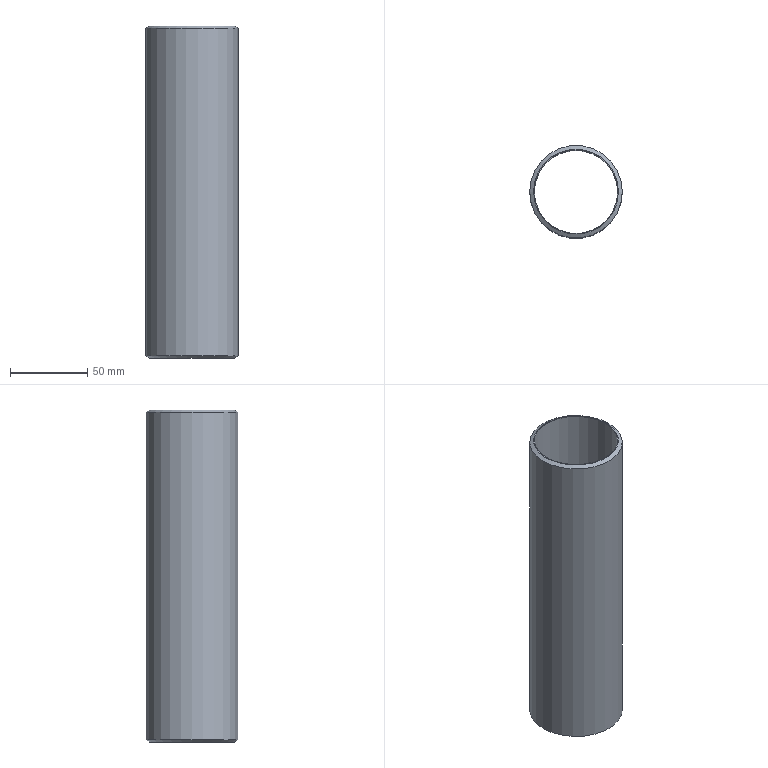Part | NX | features CHAMFER 2, CYLINDER 1, DATUM_CSYS 1, SHELL 1 | 1 solid | 6 faces | box 60 x 60 x 215 mm | volume 114839 mm3 | plane 2 | cylinder 2 | cone 2 | commonest cylinder face diameters 54 x1 60 x1
STEP:
#1=CARTESIAN_POINT('',(27.5,0.,215.));
#2=VERTEX_POINT('',#1);
#3=CARTESIAN_POINT('',(0.,0.,215.));
#4=DIRECTION('',(0.,0.,1.));
#5=DIRECTION('',(1.,0.,0.));
#6=AXIS2_PLACEMENT_3D('',#3,#4,#5);
#7=CIRCLE('',#6,27.5);
#8=EDGE_CURVE('',#2,#2,#7,.T.);
#9=ORIENTED_EDGE('',*,*,#8,.T.);
#10=EDGE_LOOP('',(#9));
#11=FACE_BOUND('',#10,.T.);
#12=CARTESIAN_POINT('',(27.,0.,215.));
#13=VERTEX_POINT('',#12);
#14=CARTESIAN_POINT('',(0.,0.,215.));
#15=DIRECTION('',(0.,0.,1.));
#16=DIRECTION('',(1.,0.,0.));
#17=AXIS2_PLACEMENT_3D('',#14,#15,#16);
#18=CIRCLE('',#17,27.);
#19=EDGE_CURVE('',#13,#13,#18,.F.);
#20=ORIENTED_EDGE('',*,*,#19,.T.);
#21=EDGE_LOOP('',(#20));
#22=FACE_BOUND('',#21,.T.);
#23=CARTESIAN_POINT('',(0.,0.,215.));
#24=DIRECTION('',(0.,0.,1.));
#25=DIRECTION('',(1.,0.,0.));
#26=AXIS2_PLACEMENT_3D('',#23,#24,#25);
#27=PLANE('',#26);
#28=ADVANCED_FACE('',(#11,#22),#27,.T.);
#29=CARTESIAN_POINT('',(-27.5,0.,0.));
#30=VERTEX_POINT('',#29);
#31=CARTESIAN_POINT('',(0.,0.,0.));
#32=DIRECTION('',(0.,0.,-1.));
#33=DIRECTION('',(-1.,0.,0.));
#34=AXIS2_PLACEMENT_3D('',#31,#32,#33);
#35=CIRCLE('',#34,27.5);
#36=EDGE_CURVE('',#30,#30,#35,.T.);
#37=ORIENTED_EDGE('',*,*,#36,.T.);
#38=EDGE_LOOP('',(#37));
#39=FACE_BOUND('',#38,.T.);
#40=CARTESIAN_POINT('',(-27.,0.,0.));
#41=VERTEX_POINT('',#40);
#42=CARTESIAN_POINT('',(0.,0.,0.));
#43=DIRECTION('',(0.,0.,-1.));
#44=DIRECTION('',(-1.,0.,0.));
#45=AXIS2_PLACEMENT_3D('',#42,#43,#44);
#46=CIRCLE('',#45,27.);
#47=EDGE_CURVE('',#41,#41,#46,.F.);
#48=ORIENTED_EDGE('',*,*,#47,.T.);
#49=EDGE_LOOP('',(#48));
#50=FACE_BOUND('',#49,.T.);
#51=CARTESIAN_POINT('',(0.,0.,0.));
#52=DIRECTION('',(0.,0.,-1.));
#53=DIRECTION('',(-1.,0.,0.));
#54=AXIS2_PLACEMENT_3D('',#51,#52,#53);
#55=PLANE('',#54);
#56=ADVANCED_FACE('',(#39,#50),#55,.T.);
#57=CARTESIAN_POINT('',(30.,0.,213.557));
#58=VERTEX_POINT('',#57);
#59=CARTESIAN_POINT('',(0.,0.,213.557));
#60=DIRECTION('',(0.,0.,1.));
#61=DIRECTION('',(1.,0.,0.));
#62=AXIS2_PLACEMENT_3D('',#59,#60,#61);
#63=CIRCLE('',#62,30.);
#64=EDGE_CURVE('',#58,#58,#63,.F.);
#65=ORIENTED_EDGE('',*,*,#64,.T.);
#66=EDGE_LOOP('',(#65));
#67=FACE_BOUND('',#66,.T.);
#68=CARTESIAN_POINT('',(-30.,0.,1.443));
#69=VERTEX_POINT('',#68);
#70=CARTESIAN_POINT('',(0.,0.,1.443));
#71=DIRECTION('',(0.,0.,-1.));
#72=DIRECTION('',(-1.,0.,0.));
#73=AXIS2_PLACEMENT_3D('',#70,#71,#72);
#74=CIRCLE('',#73,30.);
#75=EDGE_CURVE('',#69,#69,#74,.F.);
#76=ORIENTED_EDGE('',*,*,#75,.T.);
#77=EDGE_LOOP('',(#76));
#78=FACE_BOUND('',#77,.T.);
#79=CARTESIAN_POINT('',(0.,0.,0.));
#80=DIRECTION('',(0.,0.,1.));
#81=DIRECTION('',(1.,0.,0.));
#82=AXIS2_PLACEMENT_3D('',#79,#80,#81);
#83=CYLINDRICAL_SURFACE('',#82,30.);
#84=ADVANCED_FACE('',(#67,#78),#83,.T.);
#85=ORIENTED_EDGE('',*,*,#19,.F.);
#86=EDGE_LOOP('',(#85));
#87=FACE_BOUND('',#86,.T.);
#88=ORIENTED_EDGE('',*,*,#47,.F.);
#89=EDGE_LOOP('',(#88));
#90=FACE_BOUND('',#89,.T.);
#91=CARTESIAN_POINT('',(0.,0.,0.));
#92=DIRECTION('',(0.,0.,1.));
#93=DIRECTION('',(1.,0.,0.));
#94=AXIS2_PLACEMENT_3D('',#91,#92,#93);
#95=CYLINDRICAL_SURFACE('',#94,27.);
#96=ADVANCED_FACE('',(#87,#90),#95,.F.);
#97=ORIENTED_EDGE('',*,*,#36,.F.);
#98=EDGE_LOOP('',(#97));
#99=FACE_BOUND('',#98,.T.);
#100=ORIENTED_EDGE('',*,*,#75,.F.);
#101=EDGE_LOOP('',(#100));
#102=FACE_BOUND('',#101,.T.);
#103=CARTESIAN_POINT('',(0.,0.,1.443));
#104=DIRECTION('',(0.,0.,1.));
#105=DIRECTION('',(1.,0.,0.));
#106=AXIS2_PLACEMENT_3D('',#103,#104,#105);
#107=CONICAL_SURFACE('',#106,30.,1.047);
#108=ADVANCED_FACE('',(#99,#102),#107,.T.);
#109=ORIENTED_EDGE('',*,*,#8,.F.);
#110=EDGE_LOOP('',(#109));
#111=FACE_BOUND('',#110,.T.);
#112=ORIENTED_EDGE('',*,*,#64,.F.);
#113=EDGE_LOOP('',(#112));
#114=FACE_BOUND('',#113,.T.);
#115=CARTESIAN_POINT('',(0.,0.,213.557));
#116=DIRECTION('',(0.,0.,-1.));
#117=DIRECTION('',(-1.,0.,0.));
#118=AXIS2_PLACEMENT_3D('',#115,#116,#117);
#119=CONICAL_SURFACE('',#118,30.,1.047);
#120=ADVANCED_FACE('',(#111,#114),#119,.T.);
#121=CLOSED_SHELL('',(#28,#56,#84,#96,#108,#120));
#122=MANIFOLD_SOLID_BREP('',#121);
#123=(LENGTH_UNIT()NAMED_UNIT(*)SI_UNIT(.MILLI.,.METRE.));
#124=UNCERTAINTY_MEASURE_WITH_UNIT(LENGTH_MEASURE(0.00001),#123,'','');
#125=(NAMED_UNIT(*)PLANE_ANGLE_UNIT()SI_UNIT($,.RADIAN.));
#126=(NAMED_UNIT(*)SI_UNIT($,.STERADIAN.)SOLID_ANGLE_UNIT());
#127=(GEOMETRIC_REPRESENTATION_CONTEXT(3)GLOBAL_UNCERTAINTY_ASSIGNED_CONTEXT((#124))GLOBAL_UNIT_ASSIGNED_CONTEXT((#123,#125,#126))REPRESENTATION_CONTEXT('',''));
#128=ADVANCED_BREP_SHAPE_REPRESENTATION('',(#122),#127);